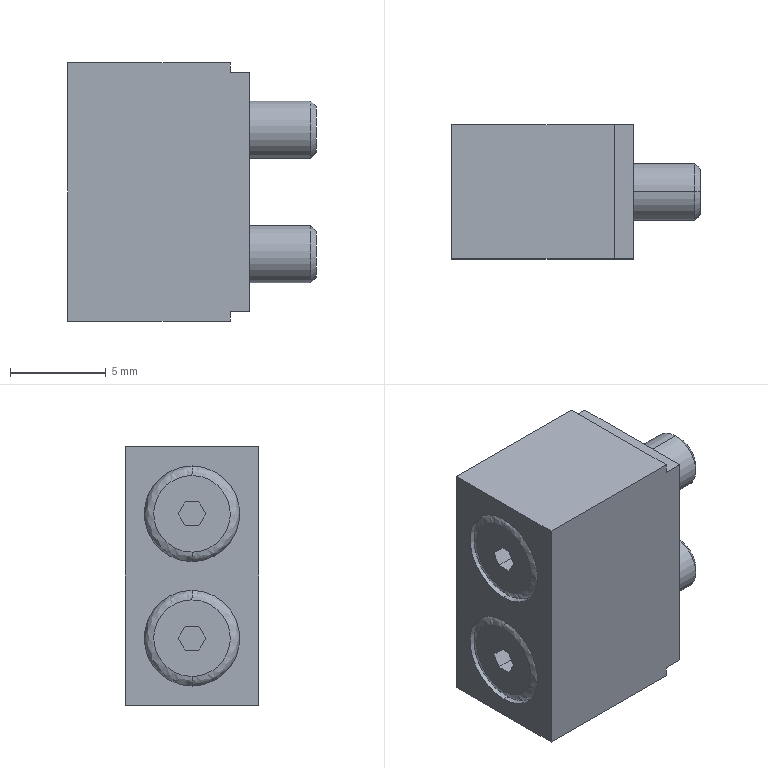Part | STEP file | QA-HI_MDX-6 B | 1 solid | 44 faces | box 13 x 7 x 13.5 mm | volume 935.094 mm3 | plane 28 | cylinder 8 | spline 4 | cone 4 | commonest cylinder face diameters 3 x4 5 x4